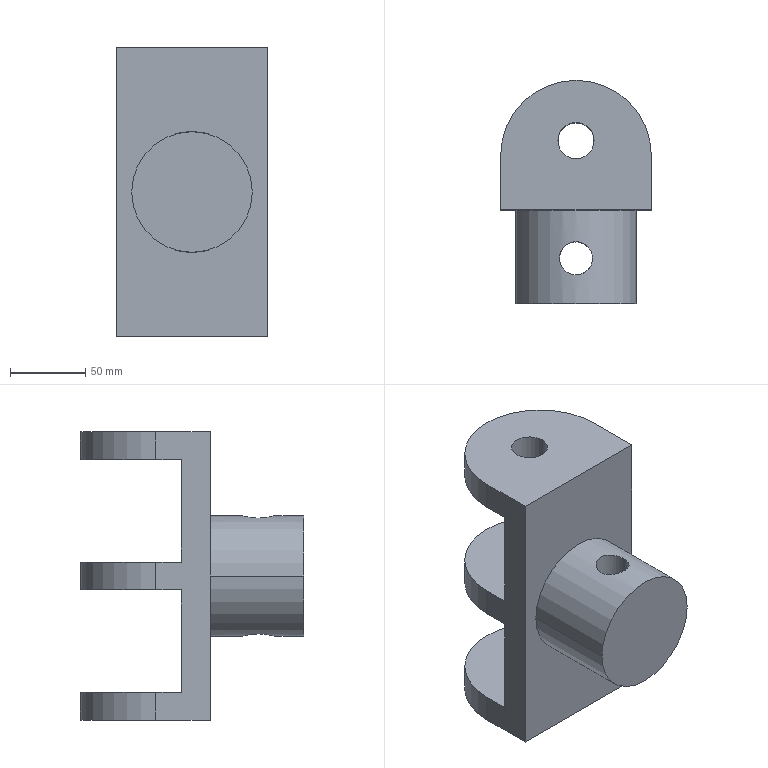Part | SolidWorks | features ICE 3, Extrusion 1 | 1 solid | 25 faces | box 100 x 148 x 191.5 mm | volume 932566 mm3 | cylinder 13 | plane 12 | commonest cylinder face diameters 24 x6 100 x3 22 x2 80 x2
STEP:
#1=CARTESIAN_POINT('',(39.,-32.,57.292));
#2=VERTEX_POINT('',#1);
#3=CARTESIAN_POINT('',(61.,-32.,57.292));
#4=VERTEX_POINT('',#3);
#5=CARTESIAN_POINT('',(39.,-32.,57.292));
#6=CARTESIAN_POINT('',(39.,-32.72,57.292));
#7=CARTESIAN_POINT('',(39.07,-33.44,57.272));
#8=CARTESIAN_POINT('',(39.356,-34.868,57.192));
#9=CARTESIAN_POINT('',(39.566,-35.556,57.134));
#10=CARTESIAN_POINT('',(39.979,-36.55,57.025));
#11=CARTESIAN_POINT('',(40.133,-36.875,56.986));
#12=CARTESIAN_POINT('',(40.474,-37.512,56.901));
#13=CARTESIAN_POINT('',(40.66,-37.823,56.855));
#14=CARTESIAN_POINT('',(41.259,-38.716,56.715));
#15=CARTESIAN_POINT('',(41.712,-39.268,56.615));
#16=CARTESIAN_POINT('',(42.472,-40.029,56.464));
#17=CARTESIAN_POINT('',(42.741,-40.273,56.413));
#18=CARTESIAN_POINT('',(43.297,-40.729,56.315));
#19=CARTESIAN_POINT('',(43.584,-40.942,56.267));
#20=CARTESIAN_POINT('',(44.474,-41.538,56.129));
#21=CARTESIAN_POINT('',(45.105,-41.877,56.045));
#22=CARTESIAN_POINT('',(46.445,-42.435,55.903));
#23=CARTESIAN_POINT('',(47.135,-42.645,55.846));
#24=CARTESIAN_POINT('',(48.192,-42.856,55.789));
#25=CARTESIAN_POINT('',(48.548,-42.91,55.775));
#26=CARTESIAN_POINT('',(49.269,-42.982,55.755));
#27=CARTESIAN_POINT('',(49.635,-43.,55.75));
#28=CARTESIAN_POINT('',(50.723,-43.,55.75));
#29=CARTESIAN_POINT('',(51.439,-42.929,55.77));
#30=CARTESIAN_POINT('',(52.501,-42.718,55.827));
#31=CARTESIAN_POINT('',(52.854,-42.63,55.85));
#32=CARTESIAN_POINT('',(53.549,-42.418,55.906));
#33=CARTESIAN_POINT('',(53.888,-42.296,55.938));
#34=CARTESIAN_POINT('',(54.883,-41.883,56.044));
#35=CARTESIAN_POINT('',(55.514,-41.545,56.127));
#36=CARTESIAN_POINT('',(56.415,-40.943,56.267));
#37=CARTESIAN_POINT('',(56.705,-40.727,56.315));
#38=CARTESIAN_POINT('',(57.259,-40.273,56.413));
#39=CARTESIAN_POINT('',(57.523,-40.033,56.463));
#40=CARTESIAN_POINT('',(58.028,-39.529,56.563));
#41=CARTESIAN_POINT('',(58.268,-39.264,56.613));
#42=CARTESIAN_POINT('',(58.724,-38.71,56.712));
#43=CARTESIAN_POINT('',(58.94,-38.419,56.761));
#44=CARTESIAN_POINT('',(59.541,-37.522,56.902));
#45=CARTESIAN_POINT('',(59.878,-36.892,56.988));
#46=CARTESIAN_POINT('',(60.43,-35.567,57.133));
#47=CARTESIAN_POINT('',(60.645,-34.866,57.192));
#48=CARTESIAN_POINT('',(60.928,-33.45,57.271));
#49=CARTESIAN_POINT('',(61.,-32.73,57.292));
#50=CARTESIAN_POINT('',(61.,-32.,57.292));
#51=B_SPLINE_CURVE_WITH_KNOTS('',3,(#5,#6,#7,#8,#9,#10,#11,#12,#13,#14,#15,#16,#17,#18,#19,#20,#21,#22,#23,#24,#25,#26,#27,#28,#29,#30,#31,#32,#33,#34,#35,#36,#37,#38,#39,#40,#41,#42,#43,#44,#45,#46,#47,#48,#49,#50),.UNSPECIFIED.,.F.,.F.,(4,2,2,2,2,2,2,2,2,2,2,2,2,2,2,2,2,2,2,2,2,2,4),(0.03456,0.03672,0.03888,0.03996,0.04104,0.04319,0.04427,0.04535,0.04751,0.04967,0.05075,0.05183,0.05399,0.05507,0.05615,0.05831,0.05939,0.06047,0.06155,0.06263,0.06479,0.06695,0.06911),.UNSPECIFIED.);
#52=EDGE_CURVE('',#2,#4,#51,.T.);
#53=ORIENTED_EDGE('',*,*,#52,.F.);
#54=CARTESIAN_POINT('',(39.,-32.,134.208));
#55=VERTEX_POINT('',#54);
#56=CARTESIAN_POINT('',(39.,-32.,-0.000012));
#57=DIRECTION('',(0.,0.,1.));
#58=VECTOR('',#57,1000.);
#59=LINE('',#56,#58);
#60=EDGE_CURVE('',#2,#55,#59,.T.);
#61=ORIENTED_EDGE('',*,*,#60,.T.);
#62=CARTESIAN_POINT('',(61.,-32.,134.208));
#63=VERTEX_POINT('',#62);
#64=CARTESIAN_POINT('',(61.,-32.,134.208));
#65=CARTESIAN_POINT('',(61.,-32.731,134.208));
#66=CARTESIAN_POINT('',(60.928,-33.448,134.229));
#67=CARTESIAN_POINT('',(60.717,-34.506,134.288));
#68=CARTESIAN_POINT('',(60.629,-34.856,134.312));
#69=CARTESIAN_POINT('',(60.418,-35.549,134.37));
#70=CARTESIAN_POINT('',(60.295,-35.892,134.403));
#71=CARTESIAN_POINT('',(59.88,-36.89,134.512));
#72=CARTESIAN_POINT('',(59.542,-37.52,134.597));
#73=CARTESIAN_POINT('',(58.943,-38.415,134.738));
#74=CARTESIAN_POINT('',(58.727,-38.706,134.787));
#75=CARTESIAN_POINT('',(58.27,-39.263,134.887));
#76=CARTESIAN_POINT('',(58.029,-39.528,134.937));
#77=CARTESIAN_POINT('',(57.272,-40.284,135.087));
#78=CARTESIAN_POINT('',(56.72,-40.739,135.186));
#79=CARTESIAN_POINT('',(55.819,-41.342,135.326));
#80=CARTESIAN_POINT('',(55.509,-41.528,135.37));
#81=CARTESIAN_POINT('',(54.877,-41.866,135.453));
#82=CARTESIAN_POINT('',(54.553,-42.02,135.491));
#83=CARTESIAN_POINT('',(53.892,-42.295,135.562));
#84=CARTESIAN_POINT('',(53.554,-42.416,135.593));
#85=CARTESIAN_POINT('',(52.863,-42.627,135.649));
#86=CARTESIAN_POINT('',(52.509,-42.716,135.673));
#87=CARTESIAN_POINT('',(51.442,-42.929,135.73));
#88=CARTESIAN_POINT('',(50.726,-43.,135.75));
#89=CARTESIAN_POINT('',(49.283,-43.,135.75));
#90=CARTESIAN_POINT('',(48.55,-42.928,135.73));
#91=CARTESIAN_POINT('',(47.136,-42.645,135.654));
#92=CARTESIAN_POINT('',(46.449,-42.436,135.598));
#93=CARTESIAN_POINT('',(45.446,-42.02,135.491));
#94=CARTESIAN_POINT('',(45.118,-41.864,135.452));
#95=CARTESIAN_POINT('',(44.484,-41.524,135.369));
#96=CARTESIAN_POINT('',(44.177,-41.339,135.325));
#97=CARTESIAN_POINT('',(43.583,-40.942,135.233));
#98=CARTESIAN_POINT('',(43.296,-40.729,135.185));
#99=CARTESIAN_POINT('',(42.742,-40.273,135.087));
#100=CARTESIAN_POINT('',(42.473,-40.03,135.036));
#101=CARTESIAN_POINT('',(41.71,-39.266,134.885));
#102=CARTESIAN_POINT('',(41.258,-38.715,134.785));
#103=CARTESIAN_POINT('',(40.661,-37.823,134.645));
#104=CARTESIAN_POINT('',(40.476,-37.515,134.6));
#105=CARTESIAN_POINT('',(40.133,-36.877,134.514));
#106=CARTESIAN_POINT('',(39.979,-36.55,134.475));
#107=CARTESIAN_POINT('',(39.565,-35.555,134.366));
#108=CARTESIAN_POINT('',(39.356,-34.869,134.308));
#109=CARTESIAN_POINT('',(39.143,-33.805,134.248));
#110=CARTESIAN_POINT('',(39.089,-33.442,134.233));
#111=CARTESIAN_POINT('',(39.018,-32.721,134.213));
#112=CARTESIAN_POINT('',(39.,-32.36,134.208));
#113=CARTESIAN_POINT('',(39.,-32.,134.208));
#114=B_SPLINE_CURVE_WITH_KNOTS('',3,(#64,#65,#66,#67,#68,#69,#70,#71,#72,#73,#74,#75,#76,#77,#78,#79,#80,#81,#82,#83,#84,#85,#86,#87,#88,#89,#90,#91,#92,#93,#94,#95,#96,#97,#98,#99,#100,#101,#102,#103,#104,#105,#106,#107,#108,#109,#110,#111,#112,#113),.UNSPECIFIED.,.F.,.F.,(4,2,2,2,2,2,2,2,2,2,2,2,2,2,2,2,2,2,2,2,2,2,2,2,4),(0.,0.00216,0.00324,0.00432,0.00648,0.00756,0.008639,0.0108,0.01188,0.01296,0.01404,0.01512,0.01728,0.01944,0.0216,0.02268,0.02376,0.02484,0.02592,0.02808,0.02916,0.03024,0.0324,0.03348,0.03456),.UNSPECIFIED.);
#115=EDGE_CURVE('',#63,#55,#114,.T.);
#116=ORIENTED_EDGE('',*,*,#115,.F.);
#117=CARTESIAN_POINT('',(61.,-32.,-0.000012));
#118=DIRECTION('',(0.,0.,1.));
#119=VECTOR('',#118,1000.);
#120=LINE('',#117,#119);
#121=EDGE_CURVE('',#4,#63,#120,.T.);
#122=ORIENTED_EDGE('',*,*,#121,.F.);
#123=EDGE_LOOP('',(#53,#61,#116,#122));
#124=FACE_OUTER_BOUND('',#123,.T.);
#125=CARTESIAN_POINT('',(50.,-32.,-0.000012));
#126=DIRECTION('',(0.,0.,1.));
#127=DIRECTION('',(1.,0.,0.));
#128=AXIS2_PLACEMENT_3D('',#125,#126,#127);
#129=CYLINDRICAL_SURFACE('',#128,11.);
#130=ADVANCED_FACE('',(#124),#129,.F.);
#131=CARTESIAN_POINT('',(38.,46.,105.));
#132=VERTEX_POINT('',#131);
#133=CARTESIAN_POINT('',(62.,46.,105.));
#134=VERTEX_POINT('',#133);
#135=CARTESIAN_POINT('',(50.,46.,105.));
#136=DIRECTION('',(0.,0.,1.));
#137=DIRECTION('',(0.,-1.,0.));
#138=AXIS2_PLACEMENT_3D('',#135,#136,#137);
#139=CIRCLE('',#138,12.);
#140=EDGE_CURVE('',#132,#134,#139,.T.);
#141=ORIENTED_EDGE('',*,*,#140,.T.);
#142=CARTESIAN_POINT('',(62.,46.,86.5));
#143=VERTEX_POINT('',#142);
#144=CARTESIAN_POINT('',(62.,46.,191.5));
#145=DIRECTION('',(0.,0.,-1.));
#146=VECTOR('',#145,1000.);
#147=LINE('',#144,#146);
#148=EDGE_CURVE('',#134,#143,#147,.T.);
#149=ORIENTED_EDGE('',*,*,#148,.T.);
#150=CARTESIAN_POINT('',(38.,46.,86.5));
#151=VERTEX_POINT('',#150);
#152=CARTESIAN_POINT('',(50.,46.,86.5));
#153=DIRECTION('',(0.,0.,-1.));
#154=DIRECTION('',(-1.,0.,0.));
#155=AXIS2_PLACEMENT_3D('',#152,#153,#154);
#156=CIRCLE('',#155,12.);
#157=EDGE_CURVE('',#143,#151,#156,.T.);
#158=ORIENTED_EDGE('',*,*,#157,.T.);
#159=CARTESIAN_POINT('',(38.,46.,191.5));
#160=DIRECTION('',(0.,0.,-1.));
#161=VECTOR('',#160,1000.);
#162=LINE('',#159,#161);
#163=EDGE_CURVE('',#132,#151,#162,.T.);
#164=ORIENTED_EDGE('',*,*,#163,.F.);
#165=EDGE_LOOP('',(#141,#149,#158,#164));
#166=FACE_OUTER_BOUND('',#165,.T.);
#167=CARTESIAN_POINT('',(50.,46.,191.5));
#168=DIRECTION('',(0.,0.,-1.));
#169=DIRECTION('',(-1.,0.,0.));
#170=AXIS2_PLACEMENT_3D('',#167,#168,#169);
#171=CYLINDRICAL_SURFACE('',#170,12.);
#172=ADVANCED_FACE('',(#166),#171,.F.);
#173=ORIENTED_EDGE('',*,*,#115,.T.);
#174=CARTESIAN_POINT('',(39.,-32.,134.208));
#175=CARTESIAN_POINT('',(39.,-31.28,134.208));
#176=CARTESIAN_POINT('',(39.07,-30.56,134.228));
#177=CARTESIAN_POINT('',(39.356,-29.132,134.308));
#178=CARTESIAN_POINT('',(39.566,-28.444,134.366));
#179=CARTESIAN_POINT('',(39.979,-27.45,134.475));
#180=CARTESIAN_POINT('',(40.133,-27.125,134.514));
#181=CARTESIAN_POINT('',(40.474,-26.488,134.599));
#182=CARTESIAN_POINT('',(40.66,-26.177,134.645));
#183=CARTESIAN_POINT('',(41.259,-25.284,134.785));
#184=CARTESIAN_POINT('',(41.712,-24.732,134.885));
#185=CARTESIAN_POINT('',(42.472,-23.971,135.036));
#186=CARTESIAN_POINT('',(42.741,-23.727,135.087));
#187=CARTESIAN_POINT('',(43.297,-23.271,135.185));
#188=CARTESIAN_POINT('',(43.584,-23.058,135.233));
#189=CARTESIAN_POINT('',(44.474,-22.462,135.371));
#190=CARTESIAN_POINT('',(45.105,-22.123,135.455));
#191=CARTESIAN_POINT('',(46.445,-21.565,135.597));
#192=CARTESIAN_POINT('',(47.135,-21.355,135.654));
#193=CARTESIAN_POINT('',(48.192,-21.144,135.711));
#194=CARTESIAN_POINT('',(48.548,-21.09,135.725));
#195=CARTESIAN_POINT('',(49.269,-21.018,135.745));
#196=CARTESIAN_POINT('',(49.635,-21.,135.75));
#197=CARTESIAN_POINT('',(50.723,-21.,135.75));
#198=CARTESIAN_POINT('',(51.439,-21.071,135.73));
#199=CARTESIAN_POINT('',(52.501,-21.282,135.673));
#200=CARTESIAN_POINT('',(52.854,-21.37,135.65));
#201=CARTESIAN_POINT('',(53.549,-21.582,135.594));
#202=CARTESIAN_POINT('',(53.888,-21.704,135.562));
#203=CARTESIAN_POINT('',(54.883,-22.117,135.456));
#204=CARTESIAN_POINT('',(55.514,-22.455,135.373));
#205=CARTESIAN_POINT('',(56.415,-23.057,135.233));
#206=CARTESIAN_POINT('',(56.705,-23.273,135.185));
#207=CARTESIAN_POINT('',(57.259,-23.727,135.087));
#208=CARTESIAN_POINT('',(57.523,-23.967,135.037));
#209=CARTESIAN_POINT('',(58.028,-24.471,134.937));
#210=CARTESIAN_POINT('',(58.268,-24.736,134.887));
#211=CARTESIAN_POINT('',(58.724,-25.29,134.788));
#212=CARTESIAN_POINT('',(58.94,-25.581,134.739));
#213=CARTESIAN_POINT('',(59.541,-26.478,134.598));
#214=CARTESIAN_POINT('',(59.878,-27.108,134.512));
#215=CARTESIAN_POINT('',(60.43,-28.433,134.367));
#216=CARTESIAN_POINT('',(60.645,-29.134,134.308));
#217=CARTESIAN_POINT('',(60.928,-30.55,134.229));
#218=CARTESIAN_POINT('',(61.,-31.27,134.208));
#219=CARTESIAN_POINT('',(61.,-32.,134.208));
#220=B_SPLINE_CURVE_WITH_KNOTS('',3,(#174,#175,#176,#177,#178,#179,#180,#181,#182,#183,#184,#185,#186,#187,#188,#189,#190,#191,#192,#193,#194,#195,#196,#197,#198,#199,#200,#201,#202,#203,#204,#205,#206,#207,#208,#209,#210,#211,#212,#213,#214,#215,#216,#217,#218,#219),.UNSPECIFIED.,.F.,.F.,(4,2,2,2,2,2,2,2,2,2,2,2,2,2,2,2,2,2,2,2,2,2,4),(0.03456,0.03672,0.03888,0.03996,0.04104,0.04319,0.04427,0.04535,0.04751,0.04967,0.05075,0.05183,0.05399,0.05507,0.05615,0.05831,0.05939,0.06047,0.06155,0.06263,0.06479,0.06695,0.06911),.UNSPECIFIED.);
#221=EDGE_CURVE('',#55,#63,#220,.T.);
#222=ORIENTED_EDGE('',*,*,#221,.T.);
#223=EDGE_LOOP('',(#173,#222));
#224=FACE_BOUND('',#223,.T.);
#225=CARTESIAN_POINT('',(90.,-62.,95.75));
#226=VERTEX_POINT('',#225);
#227=CARTESIAN_POINT('',(10.,-62.,95.75));
#228=VERTEX_POINT('',#227);
#229=CARTESIAN_POINT('',(50.,-62.,95.75));
#230=DIRECTION('',(0.,-1.,0.));
#231=DIRECTION('',(1.,0.,0.));
#232=AXIS2_PLACEMENT_3D('',#229,#230,#231);
#233=CIRCLE('',#232,40.);
#234=EDGE_CURVE('',#226,#228,#233,.T.);
#235=ORIENTED_EDGE('',*,*,#234,.F.);
#236=CARTESIAN_POINT('',(90.,0.,95.75));
#237=VERTEX_POINT('',#236);
#238=CARTESIAN_POINT('',(90.,-62.,95.75));
#239=DIRECTION('',(0.,1.,0.));
#240=VECTOR('',#239,1000.);
#241=LINE('',#238,#240);
#242=EDGE_CURVE('',#226,#237,#241,.T.);
#243=ORIENTED_EDGE('',*,*,#242,.T.);
#244=CARTESIAN_POINT('',(10.,0.,95.75));
#245=VERTEX_POINT('',#244);
#246=CARTESIAN_POINT('',(50.,0.,95.75));
#247=DIRECTION('',(0.,-1.,0.));
#248=DIRECTION('',(1.,0.,0.));
#249=AXIS2_PLACEMENT_3D('',#246,#247,#248);
#250=CIRCLE('',#249,40.);
#251=EDGE_CURVE('',#237,#245,#250,.T.);
#252=ORIENTED_EDGE('',*,*,#251,.T.);
#253=CARTESIAN_POINT('',(10.,-62.,95.75));
#254=DIRECTION('',(0.,1.,0.));
#255=VECTOR('',#254,1000.);
#256=LINE('',#253,#255);
#257=EDGE_CURVE('',#228,#245,#256,.T.);
#258=ORIENTED_EDGE('',*,*,#257,.F.);
#259=EDGE_LOOP('',(#235,#243,#252,#258));
#260=FACE_OUTER_BOUND('',#259,.T.);
#261=CARTESIAN_POINT('',(50.,-62.,95.75));
#262=DIRECTION('',(0.,1.,0.));
#263=DIRECTION('',(-1.,0.,0.));
#264=AXIS2_PLACEMENT_3D('',#261,#262,#263);
#265=CYLINDRICAL_SURFACE('',#264,40.);
#266=ADVANCED_FACE('',(#224,#260),#265,.T.);
#267=CARTESIAN_POINT('',(38.,46.,191.5));
#268=VERTEX_POINT('',#267);
#269=CARTESIAN_POINT('',(62.,46.,191.5));
#270=VERTEX_POINT('',#269);
#271=CARTESIAN_POINT('',(50.,46.,191.5));
#272=DIRECTION('',(0.,0.,1.));
#273=DIRECTION('',(1.,0.,0.));
#274=AXIS2_PLACEMENT_3D('',#271,#272,#273);
#275=CIRCLE('',#274,12.);
#276=EDGE_CURVE('',#268,#270,#275,.T.);
#277=ORIENTED_EDGE('',*,*,#276,.T.);
#278=CARTESIAN_POINT('',(62.,46.,173.));
#279=VERTEX_POINT('',#278);
#280=CARTESIAN_POINT('',(62.,46.,191.5));
#281=DIRECTION('',(0.,0.,-1.));
#282=VECTOR('',#281,1000.);
#283=LINE('',#280,#282);
#284=EDGE_CURVE('',#270,#279,#283,.T.);
#285=ORIENTED_EDGE('',*,*,#284,.T.);
#286=CARTESIAN_POINT('',(38.,46.,173.));
#287=VERTEX_POINT('',#286);
#288=CARTESIAN_POINT('',(50.,46.,173.));
#289=DIRECTION('',(0.,0.,-1.));
#290=DIRECTION('',(-1.,0.,0.));
#291=AXIS2_PLACEMENT_3D('',#288,#289,#290);
#292=CIRCLE('',#291,12.);
#293=EDGE_CURVE('',#279,#287,#292,.T.);
#294=ORIENTED_EDGE('',*,*,#293,.T.);
#295=CARTESIAN_POINT('',(38.,46.,191.5));
#296=DIRECTION('',(0.,0.,-1.));
#297=VECTOR('',#296,1000.);
#298=LINE('',#295,#297);
#299=EDGE_CURVE('',#268,#287,#298,.T.);
#300=ORIENTED_EDGE('',*,*,#299,.F.);
#301=EDGE_LOOP('',(#277,#285,#294,#300));
#302=FACE_OUTER_BOUND('',#301,.T.);
#303=CARTESIAN_POINT('',(50.,46.,191.5));
#304=DIRECTION('',(0.,0.,-1.));
#305=DIRECTION('',(-1.,0.,0.));
#306=AXIS2_PLACEMENT_3D('',#303,#304,#305);
#307=CYLINDRICAL_SURFACE('',#306,12.);
#308=ADVANCED_FACE('',(#302),#307,.F.);
#309=CARTESIAN_POINT('',(38.,46.,18.5));
#310=VERTEX_POINT('',#309);
#311=CARTESIAN_POINT('',(62.,46.,18.5));
#312=VERTEX_POINT('',#311);
#313=CARTESIAN_POINT('',(50.,46.,18.5));
#314=DIRECTION('',(0.,0.,1.));
#315=DIRECTION('',(0.,-1.,0.));
#316=AXIS2_PLACEMENT_3D('',#313,#314,#315);
#317=CIRCLE('',#316,12.);
#318=EDGE_CURVE('',#310,#312,#317,.T.);
#319=ORIENTED_EDGE('',*,*,#318,.T.);
#320=CARTESIAN_POINT('',(62.,46.,0.));
#321=VERTEX_POINT('',#320);
#322=CARTESIAN_POINT('',(62.,46.,191.5));
#323=DIRECTION('',(0.,0.,-1.));
#324=VECTOR('',#323,1000.);
#325=LINE('',#322,#324);
#326=EDGE_CURVE('',#312,#321,#325,.T.);
#327=ORIENTED_EDGE('',*,*,#326,.T.);
#328=CARTESIAN_POINT('',(38.,46.,0.));
#329=VERTEX_POINT('',#328);
#330=CARTESIAN_POINT('',(50.,46.,0.));
#331=DIRECTION('',(0.,0.,1.));
#332=DIRECTION('',(1.,0.,0.));
#333=AXIS2_PLACEMENT_3D('',#330,#331,#332);
#334=CIRCLE('',#333,12.);
#335=EDGE_CURVE('',#329,#321,#334,.T.);
#336=ORIENTED_EDGE('',*,*,#335,.F.);
#337=CARTESIAN_POINT('',(38.,46.,191.5));
#338=DIRECTION('',(0.,0.,-1.));
#339=VECTOR('',#338,1000.);
#340=LINE('',#337,#339);
#341=EDGE_CURVE('',#310,#329,#340,.T.);
#342=ORIENTED_EDGE('',*,*,#341,.F.);
#343=EDGE_LOOP('',(#319,#327,#336,#342));
#344=FACE_OUTER_BOUND('',#343,.T.);
#345=CARTESIAN_POINT('',(50.,46.,191.5));
#346=DIRECTION('',(0.,0.,-1.));
#347=DIRECTION('',(-1.,0.,0.));
#348=AXIS2_PLACEMENT_3D('',#345,#346,#347);
#349=CYLINDRICAL_SURFACE('',#348,12.);
#350=ADVANCED_FACE('',(#344),#349,.F.);
#351=CARTESIAN_POINT('',(100.,36.,86.5));
#352=VERTEX_POINT('',#351);
#353=CARTESIAN_POINT('',(100.,19.,86.5));
#354=VERTEX_POINT('',#353);
#355=CARTESIAN_POINT('',(100.,19.,86.5));
#356=DIRECTION('',(0.,-1.,0.));
#357=VECTOR('',#356,1000.);
#358=LINE('',#355,#357);
#359=EDGE_CURVE('',#352,#354,#358,.T.);
#360=ORIENTED_EDGE('',*,*,#359,.F.);
#361=CARTESIAN_POINT('',(100.,36.,105.));
#362=VERTEX_POINT('',#361);
#363=CARTESIAN_POINT('',(100.,36.,191.5));
#364=DIRECTION('',(0.,0.,-1.));
#365=VECTOR('',#364,1000.);
#366=LINE('',#363,#365);
#367=EDGE_CURVE('',#362,#352,#366,.T.);
#368=ORIENTED_EDGE('',*,*,#367,.F.);
#369=CARTESIAN_POINT('',(100.,19.,105.));
#370=VERTEX_POINT('',#369);
#371=CARTESIAN_POINT('',(100.,86.,105.));
#372=DIRECTION('',(0.,1.,0.));
#373=VECTOR('',#372,1000.);
#374=LINE('',#371,#373);
#375=EDGE_CURVE('',#370,#362,#374,.T.);
#376=ORIENTED_EDGE('',*,*,#375,.F.);
#377=CARTESIAN_POINT('',(100.,19.,173.));
#378=VERTEX_POINT('',#377);
#379=CARTESIAN_POINT('',(100.,19.,105.));
#380=DIRECTION('',(0.,0.,-1.));
#381=VECTOR('',#380,1000.);
#382=LINE('',#379,#381);
#383=EDGE_CURVE('',#378,#370,#382,.T.);
#384=ORIENTED_EDGE('',*,*,#383,.F.);
#385=CARTESIAN_POINT('',(100.,36.,173.));
#386=VERTEX_POINT('',#385);
#387=CARTESIAN_POINT('',(100.,19.,173.));
#388=DIRECTION('',(0.,-1.,0.));
#389=VECTOR('',#388,1000.);
#390=LINE('',#387,#389);
#391=EDGE_CURVE('',#386,#378,#390,.T.);
#392=ORIENTED_EDGE('',*,*,#391,.F.);
#393=CARTESIAN_POINT('',(100.,36.,191.5));
#394=VERTEX_POINT('',#393);
#395=CARTESIAN_POINT('',(100.,36.,191.5));
#396=DIRECTION('',(0.,0.,-1.));
#397=VECTOR('',#396,1000.);
#398=LINE('',#395,#397);
#399=EDGE_CURVE('',#394,#386,#398,.T.);
#400=ORIENTED_EDGE('',*,*,#399,.F.);
#401=CARTESIAN_POINT('',(100.,0.,191.5));
#402=VERTEX_POINT('',#401);
#403=CARTESIAN_POINT('',(100.,36.,191.5));
#404=DIRECTION('',(0.,1.,0.));
#405=VECTOR('',#404,1000.);
#406=LINE('',#403,#405);
#407=EDGE_CURVE('',#402,#394,#406,.T.);
#408=ORIENTED_EDGE('',*,*,#407,.F.);
#409=CARTESIAN_POINT('',(100.,0.,0.));
#410=VERTEX_POINT('',#409);
#411=CARTESIAN_POINT('',(100.,0.,191.5));
#412=DIRECTION('',(0.,0.,-1.));
#413=VECTOR('',#412,1000.);
#414=LINE('',#411,#413);
#415=EDGE_CURVE('',#402,#410,#414,.T.);
#416=ORIENTED_EDGE('',*,*,#415,.T.);
#417=CARTESIAN_POINT('',(100.,36.,0.));
#418=VERTEX_POINT('',#417);
#419=CARTESIAN_POINT('',(100.,36.,0.));
#420=DIRECTION('',(0.,1.,0.));
#421=VECTOR('',#420,1000.);
#422=LINE('',#419,#421);
#423=EDGE_CURVE('',#410,#418,#422,.T.);
#424=ORIENTED_EDGE('',*,*,#423,.T.);
#425=CARTESIAN_POINT('',(100.,36.,18.5));
#426=VERTEX_POINT('',#425);
#427=CARTESIAN_POINT('',(100.,36.,191.5));
#428=DIRECTION('',(0.,0.,-1.));
#429=VECTOR('',#428,1000.);
#430=LINE('',#427,#429);
#431=EDGE_CURVE('',#426,#418,#430,.T.);
#432=ORIENTED_EDGE('',*,*,#431,.F.);
#433=CARTESIAN_POINT('',(100.,19.,18.5));
#434=VERTEX_POINT('',#433);
#435=CARTESIAN_POINT('',(100.,86.,18.5));
#436=DIRECTION('',(0.,1.,0.));
#437=VECTOR('',#436,1000.);
#438=LINE('',#435,#437);
#439=EDGE_CURVE('',#434,#426,#438,.T.);
#440=ORIENTED_EDGE('',*,*,#439,.F.);
#441=CARTESIAN_POINT('',(100.,19.,18.5));
#442=DIRECTION('',(0.,0.,-1.));
#443=VECTOR('',#442,1000.);
#444=LINE('',#441,#443);
#445=EDGE_CURVE('',#354,#434,#444,.T.);
#446=ORIENTED_EDGE('',*,*,#445,.F.);
#447=EDGE_LOOP('',(#360,#368,#376,#384,#392,#400,#408,#416,#424,#432,#440,#446));
#448=FACE_OUTER_BOUND('',#447,.T.);
#449=CARTESIAN_POINT('',(100.,36.,191.5));
#450=DIRECTION('',(-1.,0.,0.));
#451=DIRECTION('',(0.,0.,1.));
#452=AXIS2_PLACEMENT_3D('',#449,#450,#451);
#453=PLANE('',#452);
#454=ADVANCED_FACE('',(#448),#453,.F.);
#455=CARTESIAN_POINT('',(0.,36.,86.5));
#456=VERTEX_POINT('',#455);
#457=CARTESIAN_POINT('',(50.,36.,86.5));
#458=DIRECTION('',(0.,0.,-1.));
#459=DIRECTION('',(-1.,0.,0.));
#460=AXIS2_PLACEMENT_3D('',#457,#458,#459);
#461=CIRCLE('',#460,50.);
#462=EDGE_CURVE('',#456,#352,#461,.T.);
#463=ORIENTED_EDGE('',*,*,#462,.F.);
#464=CARTESIAN_POINT('',(0.,36.,105.));
#465=VERTEX_POINT('',#464);
#466=CARTESIAN_POINT('',(0.,36.,191.5));
#467=DIRECTION('',(0.,0.,-1.));
#468=VECTOR('',#467,1000.);
#469=LINE('',#466,#468);
#470=EDGE_CURVE('',#465,#456,#469,.T.);
#471=ORIENTED_EDGE('',*,*,#470,.F.);
#472=CARTESIAN_POINT('',(50.,36.,105.));
#473=DIRECTION('',(0.,0.,1.));
#474=DIRECTION('',(0.,-1.,0.));
#475=AXIS2_PLACEMENT_3D('',#472,#473,#474);
#476=CIRCLE('',#475,50.);
#477=EDGE_CURVE('',#362,#465,#476,.T.);
#478=ORIENTED_EDGE('',*,*,#477,.F.);
#479=ORIENTED_EDGE('',*,*,#367,.T.);
#480=EDGE_LOOP('',(#463,#471,#478,#479));
#481=FACE_OUTER_BOUND('',#480,.T.);
#482=CARTESIAN_POINT('',(50.,36.,191.5));
#483=DIRECTION('',(0.,0.,-1.));
#484=DIRECTION('',(-1.,0.,0.));
#485=AXIS2_PLACEMENT_3D('',#482,#483,#484);
#486=CYLINDRICAL_SURFACE('',#485,50.);
#487=ADVANCED_FACE('',(#481),#486,.T.);
#488=CARTESIAN_POINT('',(0.,36.,18.5));
#489=VERTEX_POINT('',#488);
#490=CARTESIAN_POINT('',(50.,36.,18.5));
#491=DIRECTION('',(0.,0.,1.));
#492=DIRECTION('',(0.,-1.,0.));
#493=AXIS2_PLACEMENT_3D('',#490,#491,#492);
#494=CIRCLE('',#493,50.);
#495=EDGE_CURVE('',#426,#489,#494,.T.);
#496=ORIENTED_EDGE('',*,*,#495,.F.);
#497=ORIENTED_EDGE('',*,*,#431,.T.);
#498=CARTESIAN_POINT('',(0.,36.,0.));
#499=VERTEX_POINT('',#498);
#500=CARTESIAN_POINT('',(50.,36.,0.));
#501=DIRECTION('',(0.,0.,1.));
#502=DIRECTION('',(-1.,0.,0.));
#503=AXIS2_PLACEMENT_3D('',#500,#501,#502);
#504=CIRCLE('',#503,50.);
#505=EDGE_CURVE('',#418,#499,#504,.T.);
#506=ORIENTED_EDGE('',*,*,#505,.T.);
#507=CARTESIAN_POINT('',(0.,36.,191.5));
#508=DIRECTION('',(0.,0.,-1.));
#509=VECTOR('',#508,1000.);
#510=LINE('',#507,#509);
#511=EDGE_CURVE('',#489,#499,#510,.T.);
#512=ORIENTED_EDGE('',*,*,#511,.F.);
#513=EDGE_LOOP('',(#496,#497,#506,#512));
#514=FACE_OUTER_BOUND('',#513,.T.);
#515=CARTESIAN_POINT('',(50.,36.,191.5));
#516=DIRECTION('',(0.,0.,-1.));
#517=DIRECTION('',(-1.,0.,0.));
#518=AXIS2_PLACEMENT_3D('',#515,#516,#517);
#519=CYLINDRICAL_SURFACE('',#518,50.);
#520=ADVANCED_FACE('',(#514),#519,.T.);
#521=CARTESIAN_POINT('',(0.,36.,173.));
#522=VERTEX_POINT('',#521);
#523=CARTESIAN_POINT('',(50.,36.,173.));
#524=DIRECTION('',(0.,0.,-1.));
#525=DIRECTION('',(-1.,0.,0.));
#526=AXIS2_PLACEMENT_3D('',#523,#524,#525);
#527=CIRCLE('',#526,50.);
#528=EDGE_CURVE('',#522,#386,#527,.T.);
#529=ORIENTED_EDGE('',*,*,#528,.F.);
#530=CARTESIAN_POINT('',(0.,36.,191.5));
#531=VERTEX_POINT('',#530);
#532=CARTESIAN_POINT('',(0.,36.,191.5));
#533=DIRECTION('',(0.,0.,-1.));
#534=VECTOR('',#533,1000.);
#535=LINE('',#532,#534);
#536=EDGE_CURVE('',#531,#522,#535,.T.);
#537=ORIENTED_EDGE('',*,*,#536,.F.);
#538=CARTESIAN_POINT('',(50.,36.,191.5));
#539=DIRECTION('',(0.,0.,1.));
#540=DIRECTION('',(-1.,0.,0.));
#541=AXIS2_PLACEMENT_3D('',#538,#539,#540);
#542=CIRCLE('',#541,50.);
#543=EDGE_CURVE('',#394,#531,#542,.T.);
#544=ORIENTED_EDGE('',*,*,#543,.F.);
#545=ORIENTED_EDGE('',*,*,#399,.T.);
#546=EDGE_LOOP('',(#529,#537,#544,#545));
#547=FACE_OUTER_BOUND('',#546,.T.);
#548=CARTESIAN_POINT('',(50.,36.,191.5));
#549=DIRECTION('',(0.,0.,-1.));
#550=DIRECTION('',(-1.,0.,0.));
#551=AXIS2_PLACEMENT_3D('',#548,#549,#550);
#552=CYLINDRICAL_SURFACE('',#551,50.);
#553=ADVANCED_FACE('',(#547),#552,.T.);
#554=CARTESIAN_POINT('',(0.,19.,86.5));
#555=VERTEX_POINT('',#554);
#556=CARTESIAN_POINT('',(0.,19.,86.5));
#557=DIRECTION('',(0.,-1.,0.));
#558=VECTOR('',#557,1000.);
#559=LINE('',#556,#558);
#560=EDGE_CURVE('',#456,#555,#559,.T.);
#561=ORIENTED_EDGE('',*,*,#560,.T.);
#562=CARTESIAN_POINT('',(0.,19.,18.5));
#563=VERTEX_POINT('',#562);
#564=CARTESIAN_POINT('',(0.,19.,18.5));
#565=DIRECTION('',(0.,0.,-1.));
#566=VECTOR('',#565,1000.);
#567=LINE('',#564,#566);
#568=EDGE_CURVE('',#555,#563,#567,.T.);
#569=ORIENTED_EDGE('',*,*,#568,.T.);
#570=CARTESIAN_POINT('',(0.,86.,18.5));
#571=DIRECTION('',(0.,1.,0.));
#572=VECTOR('',#571,1000.);
#573=LINE('',#570,#572);
#574=EDGE_CURVE('',#563,#489,#573,.T.);
#575=ORIENTED_EDGE('',*,*,#574,.T.);
#576=ORIENTED_EDGE('',*,*,#511,.T.);
#577=CARTESIAN_POINT('',(0.,0.,0.));
#578=VERTEX_POINT('',#577);
#579=CARTESIAN_POINT('',(0.,0.,0.));
#580=DIRECTION('',(0.,-1.,0.));
#581=VECTOR('',#580,1000.);
#582=LINE('',#579,#581);
#583=EDGE_CURVE('',#499,#578,#582,.T.);
#584=ORIENTED_EDGE('',*,*,#583,.T.);
#585=CARTESIAN_POINT('',(0.,0.,191.5));
#586=VERTEX_POINT('',#585);
#587=CARTESIAN_POINT('',(0.,0.,191.5));
#588=DIRECTION('',(0.,0.,-1.));
#589=VECTOR('',#588,1000.);
#590=LINE('',#587,#589);
#591=EDGE_CURVE('',#586,#578,#590,.T.);
#592=ORIENTED_EDGE('',*,*,#591,.F.);
#593=CARTESIAN_POINT('',(0.,0.,191.5));
#594=DIRECTION('',(0.,-1.,0.));
#595=VECTOR('',#594,1000.);
#596=LINE('',#593,#595);
#597=EDGE_CURVE('',#531,#586,#596,.T.);
#598=ORIENTED_EDGE('',*,*,#597,.F.);
#599=ORIENTED_EDGE('',*,*,#536,.T.);
#600=CARTESIAN_POINT('',(0.,19.,173.));
#601=VERTEX_POINT('',#600);
#602=CARTESIAN_POINT('',(0.,19.,173.));
#603=DIRECTION('',(0.,-1.,0.));
#604=VECTOR('',#603,1000.);
#605=LINE('',#602,#604);
#606=EDGE_CURVE('',#522,#601,#605,.T.);
#607=ORIENTED_EDGE('',*,*,#606,.T.);
#608=CARTESIAN_POINT('',(0.,19.,105.));
#609=VERTEX_POINT('',#608);
#610=CARTESIAN_POINT('',(0.,19.,105.));
#611=DIRECTION('',(0.,0.,-1.));
#612=VECTOR('',#611,1000.);
#613=LINE('',#610,#612);
#614=EDGE_CURVE('',#601,#609,#613,.T.);
#615=ORIENTED_EDGE('',*,*,#614,.T.);
#616=CARTESIAN_POINT('',(0.,86.,105.));
#617=DIRECTION('',(0.,1.,0.));
#618=VECTOR('',#617,1000.);
#619=LINE('',#616,#618);
#620=EDGE_CURVE('',#609,#465,#619,.T.);
#621=ORIENTED_EDGE('',*,*,#620,.T.);
#622=ORIENTED_EDGE('',*,*,#470,.T.);
#623=EDGE_LOOP('',(#561,#569,#575,#576,#584,#592,#598,#599,#607,#615,#621,#622));
#624=FACE_OUTER_BOUND('',#623,.T.);
#625=CARTESIAN_POINT('',(0.,0.,191.5));
#626=DIRECTION('',(1.,0.,0.));
#627=DIRECTION('',(0.,0.,-1.));
#628=AXIS2_PLACEMENT_3D('',#625,#626,#627);
#629=PLANE('',#628);
#630=ADVANCED_FACE('',(#624),#629,.F.);
#631=ORIENTED_EDGE('',*,*,#326,.F.);
#632=CARTESIAN_POINT('',(50.,46.,18.5));
#633=DIRECTION('',(0.,0.,1.));
#634=DIRECTION('',(0.,-1.,0.));
#635=AXIS2_PLACEMENT_3D('',#632,#633,#634);
#636=CIRCLE('',#635,12.);
#637=EDGE_CURVE('',#312,#310,#636,.T.);
#638=ORIENTED_EDGE('',*,*,#637,.T.);
#639=ORIENTED_EDGE('',*,*,#341,.T.);
#640=CARTESIAN_POINT('',(50.,46.,0.));
#641=DIRECTION('',(0.,0.,1.));
#642=DIRECTION('',(1.,0.,0.));
#643=AXIS2_PLACEMENT_3D('',#640,#641,#642);
#644=CIRCLE('',#643,12.);
#645=EDGE_CURVE('',#321,#329,#644,.T.);
#646=ORIENTED_EDGE('',*,*,#645,.F.);
#647=EDGE_LOOP('',(#631,#638,#639,#646));
#648=FACE_OUTER_BOUND('',#647,.T.);
#649=CARTESIAN_POINT('',(50.,46.,191.5));
#650=DIRECTION('',(0.,0.,-1.));
#651=DIRECTION('',(-1.,0.,0.));
#652=AXIS2_PLACEMENT_3D('',#649,#650,#651);
#653=CYLINDRICAL_SURFACE('',#652,12.);
#654=ADVANCED_FACE('',(#648),#653,.F.);
#655=ORIENTED_EDGE('',*,*,#284,.F.);
#656=CARTESIAN_POINT('',(50.,46.,191.5));
#657=DIRECTION('',(0.,0.,1.));
#658=DIRECTION('',(1.,0.,0.));
#659=AXIS2_PLACEMENT_3D('',#656,#657,#658);
#660=CIRCLE('',#659,12.);
#661=EDGE_CURVE('',#270,#268,#660,.T.);
#662=ORIENTED_EDGE('',*,*,#661,.T.);
#663=ORIENTED_EDGE('',*,*,#299,.T.);
#664=CARTESIAN_POINT('',(50.,46.,173.));
#665=DIRECTION('',(0.,0.,-1.));
#666=DIRECTION('',(-1.,0.,0.));
#667=AXIS2_PLACEMENT_3D('',#664,#665,#666);
#668=CIRCLE('',#667,12.);
#669=EDGE_CURVE('',#287,#279,#668,.T.);
#670=ORIENTED_EDGE('',*,*,#669,.T.);
#671=EDGE_LOOP('',(#655,#662,#663,#670));
#672=FACE_OUTER_BOUND('',#671,.T.);
#673=CARTESIAN_POINT('',(50.,46.,191.5));
#674=DIRECTION('',(0.,0.,-1.));
#675=DIRECTION('',(-1.,0.,0.));
#676=AXIS2_PLACEMENT_3D('',#673,#674,#675);
#677=CYLINDRICAL_SURFACE('',#676,12.);
#678=ADVANCED_FACE('',(#672),#677,.F.);
#679=CARTESIAN_POINT('',(100.,0.,191.5));
#680=DIRECTION('',(1.,0.,0.));
#681=VECTOR('',#680,1000.);
#682=LINE('',#679,#681);
#683=EDGE_CURVE('',#586,#402,#682,.T.);
#684=ORIENTED_EDGE('',*,*,#683,.T.);
#685=ORIENTED_EDGE('',*,*,#407,.T.);
#686=ORIENTED_EDGE('',*,*,#543,.T.);
#687=ORIENTED_EDGE('',*,*,#597,.T.);
#688=EDGE_LOOP('',(#684,#685,#686,#687));
#689=FACE_OUTER_BOUND('',#688,.T.);
#690=ORIENTED_EDGE('',*,*,#276,.F.);
#691=ORIENTED_EDGE('',*,*,#661,.F.);
#692=EDGE_LOOP('',(#690,#691));
#693=FACE_BOUND('',#692,.T.);
#694=CARTESIAN_POINT('',(50.,36.,191.5));
#695=DIRECTION('',(0.,0.,-1.));
#696=DIRECTION('',(-1.,0.,0.));
#697=AXIS2_PLACEMENT_3D('',#694,#695,#696);
#698=PLANE('',#697);
#699=ADVANCED_FACE('',(#689,#693),#698,.F.);
#700=CARTESIAN_POINT('',(100.,0.,0.));
#701=DIRECTION('',(1.,0.,0.));
#702=VECTOR('',#701,1000.);
#703=LINE('',#700,#702);
#704=EDGE_CURVE('',#578,#410,#703,.T.);
#705=ORIENTED_EDGE('',*,*,#704,.F.);
#706=ORIENTED_EDGE('',*,*,#583,.F.);
#707=ORIENTED_EDGE('',*,*,#505,.F.);
#708=ORIENTED_EDGE('',*,*,#423,.F.);
#709=EDGE_LOOP('',(#705,#706,#707,#708));
#710=FACE_OUTER_BOUND('',#709,.T.);
#711=ORIENTED_EDGE('',*,*,#335,.T.);
#712=ORIENTED_EDGE('',*,*,#645,.T.);
#713=EDGE_LOOP('',(#711,#712));
#714=FACE_BOUND('',#713,.T.);
#715=CARTESIAN_POINT('',(50.,36.,0.));
#716=DIRECTION('',(0.,0.,-1.));
#717=DIRECTION('',(-1.,0.,0.));
#718=AXIS2_PLACEMENT_3D('',#715,#716,#717);
#719=PLANE('',#718);
#720=ADVANCED_FACE('',(#710,#714),#719,.T.);
#721=CARTESIAN_POINT('',(50.,0.,95.75));
#722=DIRECTION('',(0.,-1.,0.));
#723=DIRECTION('',(1.,0.,0.));
#724=AXIS2_PLACEMENT_3D('',#721,#722,#723);
#725=CIRCLE('',#724,40.);
#726=EDGE_CURVE('',#245,#237,#725,.T.);
#727=ORIENTED_EDGE('',*,*,#726,.F.);
#728=ORIENTED_EDGE('',*,*,#251,.F.);
#729=EDGE_LOOP('',(#727,#728));
#730=FACE_BOUND('',#729,.T.);
#731=ORIENTED_EDGE('',*,*,#704,.T.);
#732=ORIENTED_EDGE('',*,*,#415,.F.);
#733=ORIENTED_EDGE('',*,*,#683,.F.);
#734=ORIENTED_EDGE('',*,*,#591,.T.);
#735=EDGE_LOOP('',(#731,#732,#733,#734));
#736=FACE_OUTER_BOUND('',#735,.T.);
#737=CARTESIAN_POINT('',(100.,0.,191.5));
#738=DIRECTION('',(0.,1.,0.));
#739=DIRECTION('',(-1.,0.,0.));
#740=AXIS2_PLACEMENT_3D('',#737,#738,#739);
#741=PLANE('',#740);
#742=ADVANCED_FACE('',(#730,#736),#741,.F.);
#743=ORIENTED_EDGE('',*,*,#242,.F.);
#744=CARTESIAN_POINT('',(50.,-62.,95.75));
#745=DIRECTION('',(0.,-1.,0.));
#746=DIRECTION('',(1.,0.,0.));
#747=AXIS2_PLACEMENT_3D('',#744,#745,#746);
#748=CIRCLE('',#747,40.);
#749=EDGE_CURVE('',#228,#226,#748,.T.);
#750=ORIENTED_EDGE('',*,*,#749,.F.);
#751=ORIENTED_EDGE('',*,*,#257,.T.);
#752=ORIENTED_EDGE('',*,*,#726,.T.);
#753=EDGE_LOOP('',(#743,#750,#751,#752));
#754=FACE_OUTER_BOUND('',#753,.T.);
#755=CARTESIAN_POINT('',(61.,-32.,57.292));
#756=CARTESIAN_POINT('',(61.,-31.269,57.292));
#757=CARTESIAN_POINT('',(60.928,-30.552,57.271));
#758=CARTESIAN_POINT('',(60.717,-29.494,57.212));
#759=CARTESIAN_POINT('',(60.629,-29.144,57.188));
#760=CARTESIAN_POINT('',(60.418,-28.451,57.13));
#761=CARTESIAN_POINT('',(60.295,-28.108,57.097));
#762=CARTESIAN_POINT('',(59.88,-27.11,56.988));
#763=CARTESIAN_POINT('',(59.542,-26.48,56.903));
#764=CARTESIAN_POINT('',(58.943,-25.585,56.762));
#765=CARTESIAN_POINT('',(58.727,-25.294,56.713));
#766=CARTESIAN_POINT('',(58.27,-24.737,56.613));
#767=CARTESIAN_POINT('',(58.029,-24.472,56.563));
#768=CARTESIAN_POINT('',(57.272,-23.716,56.413));
#769=CARTESIAN_POINT('',(56.72,-23.261,56.314));
#770=CARTESIAN_POINT('',(55.819,-22.658,56.174));
#771=CARTESIAN_POINT('',(55.509,-22.472,56.13));
#772=CARTESIAN_POINT('',(54.877,-22.134,56.047));
#773=CARTESIAN_POINT('',(54.553,-21.98,56.009));
#774=CARTESIAN_POINT('',(53.892,-21.705,55.938));
#775=CARTESIAN_POINT('',(53.554,-21.584,55.907));
#776=CARTESIAN_POINT('',(52.863,-21.373,55.851));
#777=CARTESIAN_POINT('',(52.509,-21.284,55.827));
#778=CARTESIAN_POINT('',(51.442,-21.071,55.77));
#779=CARTESIAN_POINT('',(50.726,-21.,55.75));
#780=CARTESIAN_POINT('',(49.283,-21.,55.75));
#781=CARTESIAN_POINT('',(48.55,-21.072,55.77));
#782=CARTESIAN_POINT('',(47.136,-21.355,55.846));
#783=CARTESIAN_POINT('',(46.449,-21.564,55.902));
#784=CARTESIAN_POINT('',(45.446,-21.98,56.009));
#785=CARTESIAN_POINT('',(45.118,-22.136,56.048));
#786=CARTESIAN_POINT('',(44.484,-22.476,56.131));
#787=CARTESIAN_POINT('',(44.177,-22.661,56.175));
#788=CARTESIAN_POINT('',(43.583,-23.058,56.267));
#789=CARTESIAN_POINT('',(43.296,-23.271,56.315));
#790=CARTESIAN_POINT('',(42.742,-23.727,56.413));
#791=CARTESIAN_POINT('',(42.473,-23.97,56.464));
#792=CARTESIAN_POINT('',(41.71,-24.734,56.615));
#793=CARTESIAN_POINT('',(41.258,-25.285,56.715));
#794=CARTESIAN_POINT('',(40.661,-26.177,56.855));
#795=CARTESIAN_POINT('',(40.476,-26.485,56.9));
#796=CARTESIAN_POINT('',(40.133,-27.123,56.986));
#797=CARTESIAN_POINT('',(39.979,-27.45,57.025));
#798=CARTESIAN_POINT('',(39.565,-28.445,57.134));
#799=CARTESIAN_POINT('',(39.356,-29.131,57.192));
#800=CARTESIAN_POINT('',(39.143,-30.195,57.252));
#801=CARTESIAN_POINT('',(39.089,-30.558,57.267));
#802=CARTESIAN_POINT('',(39.018,-31.279,57.287));
#803=CARTESIAN_POINT('',(39.,-31.64,57.292));
#804=CARTESIAN_POINT('',(39.,-32.,57.292));
#805=B_SPLINE_CURVE_WITH_KNOTS('',3,(#755,#756,#757,#758,#759,#760,#761,#762,#763,#764,#765,#766,#767,#768,#769,#770,#771,#772,#773,#774,#775,#776,#777,#778,#779,#780,#781,#782,#783,#784,#785,#786,#787,#788,#789,#790,#791,#792,#793,#794,#795,#796,#797,#798,#799,#800,#801,#802,#803,#804),.UNSPECIFIED.,.F.,.F.,(4,2,2,2,2,2,2,2,2,2,2,2,2,2,2,2,2,2,2,2,2,2,2,2,4),(0.,0.00216,0.00324,0.00432,0.00648,0.00756,0.008639,0.0108,0.01188,0.01296,0.01404,0.01512,0.01728,0.01944,0.0216,0.02268,0.02376,0.02484,0.02592,0.02808,0.02916,0.03024,0.0324,0.03348,0.03456),.UNSPECIFIED.);
#806=EDGE_CURVE('',#4,#2,#805,.T.);
#807=ORIENTED_EDGE('',*,*,#806,.T.);
#808=ORIENTED_EDGE('',*,*,#52,.T.);
#809=EDGE_LOOP('',(#807,#808));
#810=FACE_BOUND('',#809,.T.);
#811=CARTESIAN_POINT('',(50.,-62.,95.75));
#812=DIRECTION('',(0.,1.,0.));
#813=DIRECTION('',(-1.,0.,0.));
#814=AXIS2_PLACEMENT_3D('',#811,#812,#813);
#815=CYLINDRICAL_SURFACE('',#814,40.);
#816=ADVANCED_FACE('',(#754,#810),#815,.T.);
#817=ORIENTED_EDGE('',*,*,#749,.T.);
#818=ORIENTED_EDGE('',*,*,#234,.T.);
#819=EDGE_LOOP('',(#817,#818));
#820=FACE_OUTER_BOUND('',#819,.T.);
#821=CARTESIAN_POINT('',(50.,-62.,95.75));
#822=DIRECTION('',(0.,-1.,0.));
#823=DIRECTION('',(1.,0.,0.));
#824=AXIS2_PLACEMENT_3D('',#821,#822,#823);
#825=PLANE('',#824);
#826=ADVANCED_FACE('',(#820),#825,.T.);
#827=ORIENTED_EDGE('',*,*,#669,.F.);
#828=ORIENTED_EDGE('',*,*,#293,.F.);
#829=EDGE_LOOP('',(#827,#828));
#830=FACE_BOUND('',#829,.T.);
#831=ORIENTED_EDGE('',*,*,#528,.T.);
#832=ORIENTED_EDGE('',*,*,#391,.T.);
#833=CARTESIAN_POINT('',(100.,19.,173.));
#834=DIRECTION('',(-1.,0.,0.));
#835=VECTOR('',#834,1000.);
#836=LINE('',#833,#835);
#837=EDGE_CURVE('',#378,#601,#836,.T.);
#838=ORIENTED_EDGE('',*,*,#837,.T.);
#839=ORIENTED_EDGE('',*,*,#606,.F.);
#840=EDGE_LOOP('',(#831,#832,#838,#839));
#841=FACE_OUTER_BOUND('',#840,.T.);
#842=CARTESIAN_POINT('',(100.,19.,173.));
#843=DIRECTION('',(0.,0.,-1.));
#844=DIRECTION('',(-1.,0.,0.));
#845=AXIS2_PLACEMENT_3D('',#842,#843,#844);
#846=PLANE('',#845);
#847=ADVANCED_FACE('',(#830,#841),#846,.T.);
#848=ORIENTED_EDGE('',*,*,#140,.F.);
#849=CARTESIAN_POINT('',(50.,46.,105.));
#850=DIRECTION('',(0.,0.,1.));
#851=DIRECTION('',(0.,-1.,0.));
#852=AXIS2_PLACEMENT_3D('',#849,#850,#851);
#853=CIRCLE('',#852,12.);
#854=EDGE_CURVE('',#134,#132,#853,.T.);
#855=ORIENTED_EDGE('',*,*,#854,.F.);
#856=EDGE_LOOP('',(#848,#855));
#857=FACE_BOUND('',#856,.T.);
#858=ORIENTED_EDGE('',*,*,#477,.T.);
#859=ORIENTED_EDGE('',*,*,#620,.F.);
#860=CARTESIAN_POINT('',(100.,19.,105.));
#861=DIRECTION('',(-1.,0.,0.));
#862=VECTOR('',#861,1000.);
#863=LINE('',#860,#862);
#864=EDGE_CURVE('',#370,#609,#863,.T.);
#865=ORIENTED_EDGE('',*,*,#864,.F.);
#866=ORIENTED_EDGE('',*,*,#375,.T.);
#867=EDGE_LOOP('',(#858,#859,#865,#866));
#868=FACE_OUTER_BOUND('',#867,.T.);
#869=CARTESIAN_POINT('',(100.,86.,105.));
#870=DIRECTION('',(0.,0.,1.));
#871=DIRECTION('',(0.,-1.,0.));
#872=AXIS2_PLACEMENT_3D('',#869,#870,#871);
#873=PLANE('',#872);
#874=ADVANCED_FACE('',(#857,#868),#873,.T.);
#875=ORIENTED_EDGE('',*,*,#614,.F.);
#876=ORIENTED_EDGE('',*,*,#837,.F.);
#877=ORIENTED_EDGE('',*,*,#383,.T.);
#878=ORIENTED_EDGE('',*,*,#864,.T.);
#879=EDGE_LOOP('',(#875,#876,#877,#878));
#880=FACE_OUTER_BOUND('',#879,.T.);
#881=CARTESIAN_POINT('',(100.,19.,105.));
#882=DIRECTION('',(0.,1.,0.));
#883=DIRECTION('',(0.,0.,1.));
#884=AXIS2_PLACEMENT_3D('',#881,#882,#883);
#885=PLANE('',#884);
#886=ADVANCED_FACE('',(#880),#885,.T.);
#887=CARTESIAN_POINT('',(50.,46.,86.5));
#888=DIRECTION('',(0.,0.,-1.));
#889=DIRECTION('',(-1.,0.,0.));
#890=AXIS2_PLACEMENT_3D('',#887,#888,#889);
#891=CIRCLE('',#890,12.);
#892=EDGE_CURVE('',#151,#143,#891,.T.);
#893=ORIENTED_EDGE('',*,*,#892,.F.);
#894=ORIENTED_EDGE('',*,*,#157,.F.);
#895=EDGE_LOOP('',(#893,#894));
#896=FACE_BOUND('',#895,.T.);
#897=ORIENTED_EDGE('',*,*,#462,.T.);
#898=ORIENTED_EDGE('',*,*,#359,.T.);
#899=CARTESIAN_POINT('',(100.,19.,86.5));
#900=DIRECTION('',(-1.,0.,0.));
#901=VECTOR('',#900,1000.);
#902=LINE('',#899,#901);
#903=EDGE_CURVE('',#354,#555,#902,.T.);
#904=ORIENTED_EDGE('',*,*,#903,.T.);
#905=ORIENTED_EDGE('',*,*,#560,.F.);
#906=EDGE_LOOP('',(#897,#898,#904,#905));
#907=FACE_OUTER_BOUND('',#906,.T.);
#908=CARTESIAN_POINT('',(100.,19.,86.5));
#909=DIRECTION('',(0.,0.,-1.));
#910=DIRECTION('',(-1.,0.,0.));
#911=AXIS2_PLACEMENT_3D('',#908,#909,#910);
#912=PLANE('',#911);
#913=ADVANCED_FACE('',(#896,#907),#912,.T.);
#914=ORIENTED_EDGE('',*,*,#318,.F.);
#915=ORIENTED_EDGE('',*,*,#637,.F.);
#916=EDGE_LOOP('',(#914,#915));
#917=FACE_BOUND('',#916,.T.);
#918=ORIENTED_EDGE('',*,*,#495,.T.);
#919=ORIENTED_EDGE('',*,*,#574,.F.);
#920=CARTESIAN_POINT('',(100.,19.,18.5));
#921=DIRECTION('',(-1.,0.,0.));
#922=VECTOR('',#921,1000.);
#923=LINE('',#920,#922);
#924=EDGE_CURVE('',#434,#563,#923,.T.);
#925=ORIENTED_EDGE('',*,*,#924,.F.);
#926=ORIENTED_EDGE('',*,*,#439,.T.);
#927=EDGE_LOOP('',(#918,#919,#925,#926));
#928=FACE_OUTER_BOUND('',#927,.T.);
#929=CARTESIAN_POINT('',(100.,86.,18.5));
#930=DIRECTION('',(0.,0.,1.));
#931=DIRECTION('',(0.,-1.,0.));
#932=AXIS2_PLACEMENT_3D('',#929,#930,#931);
#933=PLANE('',#932);
#934=ADVANCED_FACE('',(#917,#928),#933,.T.);
#935=ORIENTED_EDGE('',*,*,#568,.F.);
#936=ORIENTED_EDGE('',*,*,#903,.F.);
#937=ORIENTED_EDGE('',*,*,#445,.T.);
#938=ORIENTED_EDGE('',*,*,#924,.T.);
#939=EDGE_LOOP('',(#935,#936,#937,#938));
#940=FACE_OUTER_BOUND('',#939,.T.);
#941=CARTESIAN_POINT('',(100.,19.,18.5));
#942=DIRECTION('',(0.,1.,0.));
#943=DIRECTION('',(0.,0.,1.));
#944=AXIS2_PLACEMENT_3D('',#941,#942,#943);
#945=PLANE('',#944);
#946=ADVANCED_FACE('',(#940),#945,.T.);
#947=ORIENTED_EDGE('',*,*,#148,.F.);
#948=ORIENTED_EDGE('',*,*,#854,.T.);
#949=ORIENTED_EDGE('',*,*,#163,.T.);
#950=ORIENTED_EDGE('',*,*,#892,.T.);
#951=EDGE_LOOP('',(#947,#948,#949,#950));
#952=FACE_OUTER_BOUND('',#951,.T.);
#953=CARTESIAN_POINT('',(50.,46.,191.5));
#954=DIRECTION('',(0.,0.,-1.));
#955=DIRECTION('',(-1.,0.,0.));
#956=AXIS2_PLACEMENT_3D('',#953,#954,#955);
#957=CYLINDRICAL_SURFACE('',#956,12.);
#958=ADVANCED_FACE('',(#952),#957,.F.);
#959=ORIENTED_EDGE('',*,*,#60,.F.);
#960=ORIENTED_EDGE('',*,*,#806,.F.);
#961=ORIENTED_EDGE('',*,*,#121,.T.);
#962=ORIENTED_EDGE('',*,*,#221,.F.);
#963=EDGE_LOOP('',(#959,#960,#961,#962));
#964=FACE_OUTER_BOUND('',#963,.T.);
#965=CARTESIAN_POINT('',(50.,-32.,-0.000012));
#966=DIRECTION('',(0.,0.,1.));
#967=DIRECTION('',(1.,0.,0.));
#968=AXIS2_PLACEMENT_3D('',#965,#966,#967);
#969=CYLINDRICAL_SURFACE('',#968,11.);
#970=ADVANCED_FACE('',(#964),#969,.F.);
#971=CLOSED_SHELL('',(#130,#172,#266,#308,#350,#454,#487,#520,#553,#630,#654,#678,#699,#720,#742,#816,#826,#847,#874,#886,#913,#934,#946,#958,#970));
#972=MANIFOLD_SOLID_BREP('',#971);
#973=CARTESIAN_POINT('',(0.,0.,0.));
#974=DIRECTION('',(0.,0.,1.));
#975=DIRECTION('',(1.,0.,0.));
#976=AXIS2_PLACEMENT_3D('',#973,#974,#975);
#977=(LENGTH_UNIT()NAMED_UNIT(*)SI_UNIT(.MILLI.,.METRE.));
#978=UNCERTAINTY_MEASURE_WITH_UNIT(LENGTH_MEASURE(0.00001),#977,'','');
#979=(NAMED_UNIT(*)PLANE_ANGLE_UNIT()SI_UNIT($,.RADIAN.));
#980=(NAMED_UNIT(*)SI_UNIT($,.STERADIAN.)SOLID_ANGLE_UNIT());
#981=(GEOMETRIC_REPRESENTATION_CONTEXT(3)GLOBAL_UNCERTAINTY_ASSIGNED_CONTEXT((#978))GLOBAL_UNIT_ASSIGNED_CONTEXT((#977,#979,#980))REPRESENTATION_CONTEXT('',''));
#982=ADVANCED_BREP_SHAPE_REPRESENTATION('',(#972,#976),#981);